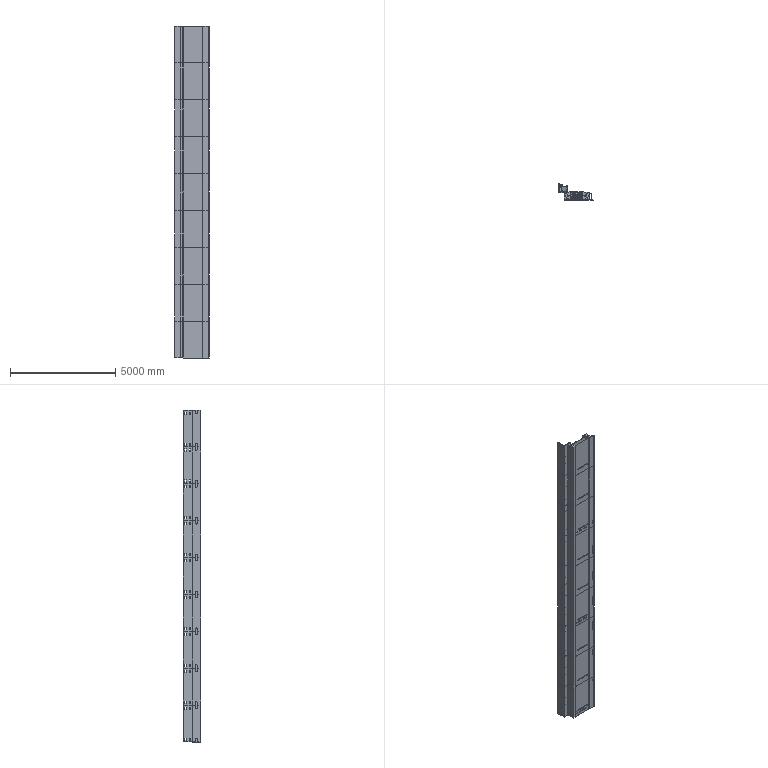Part | SolidWorks | 246 solids | 8046 faces | volume 3123900816 mm3 | plane 4506 | cylinder 1458 | spline 1146 | cone 648 | torus 216 | sphere 72 | commonest cylinder face diameters 10 x450 80 x234 25 x126 33 x126 70 x126 50 x108